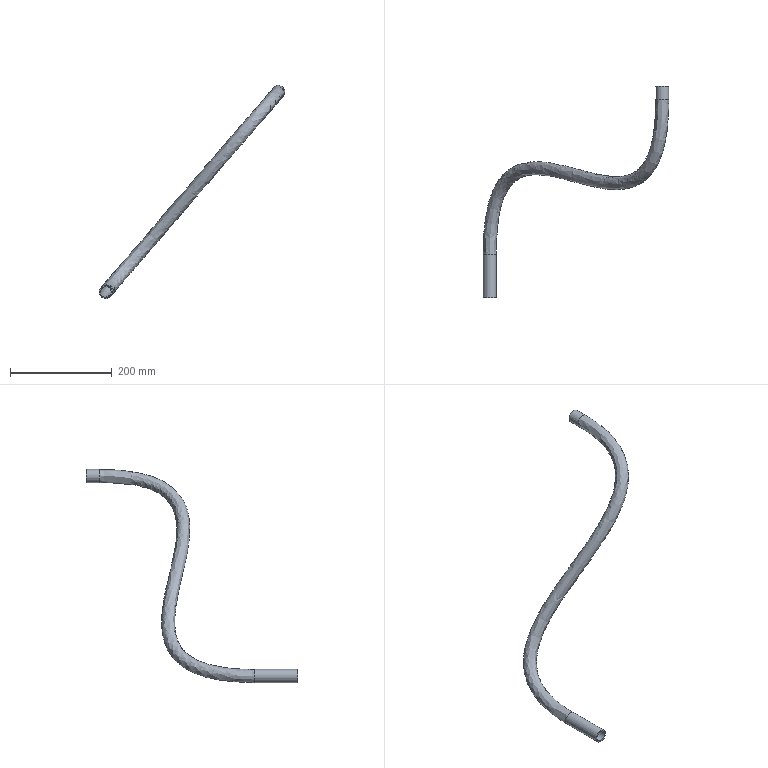Part | STEP file | Part 9^JBJ-F-0000-00 | 1 solid | 8 faces | box 365.356 x 414.992 x 419.382 mm | volume 128951 mm3 | cylinder 4 | spline 2 | plane 2 | commonest cylinder face diameters 22 x2 26 x2